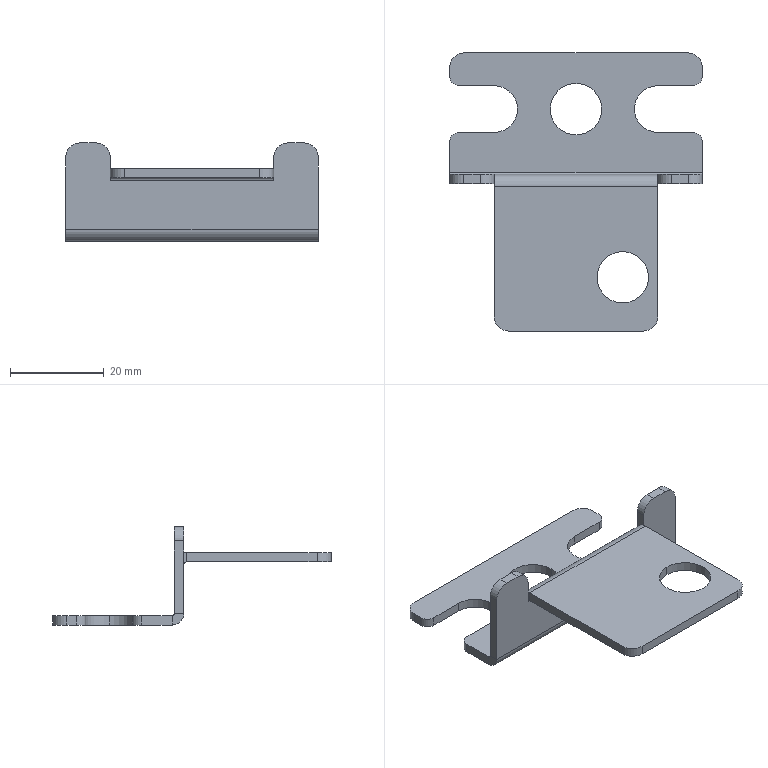Part | SolidWorks | features Fillet 3, EdgeFlange 2, ICE 2, Cut 1, FlatPattern 1, SMBaseFlange 1, SheetMetal 1 | 1 solid | 51 faces | box 54 x 59.5 x 21 mm | volume 5826 mm3 | plane 28 | cylinder 23 | commonest cylinder face diameters 6 x8 4 x4 11 x4 10 x3 1 x2 5 x2
STEP:
#1=CARTESIAN_POINT('',(10.,-28.5,13.5));
#2=VERTEX_POINT('',#1);
#3=CARTESIAN_POINT('',(10.,-39.5,13.5));
#4=VERTEX_POINT('',#3);
#5=CARTESIAN_POINT('',(10.,-34.,13.5));
#6=DIRECTION('',(0.,0.,1.));
#7=DIRECTION('',(0.,-1.,0.));
#8=AXIS2_PLACEMENT_3D('',#5,#6,#7);
#9=CIRCLE('',#8,5.5);
#10=EDGE_CURVE('',#2,#4,#9,.T.);
#11=ORIENTED_EDGE('',*,*,#10,.T.);
#12=CARTESIAN_POINT('',(10.,-39.5,11.5));
#13=VERTEX_POINT('',#12);
#14=CARTESIAN_POINT('',(10.,-39.5,21.5));
#15=DIRECTION('',(0.,0.,-1.));
#16=VECTOR('',#15,1000.);
#17=LINE('',#14,#16);
#18=EDGE_CURVE('',#4,#13,#17,.T.);
#19=ORIENTED_EDGE('',*,*,#18,.T.);
#20=CARTESIAN_POINT('',(10.,-28.5,11.5));
#21=VERTEX_POINT('',#20);
#22=CARTESIAN_POINT('',(10.,-34.,11.5));
#23=DIRECTION('',(0.,0.,-1.));
#24=DIRECTION('',(0.,1.,0.));
#25=AXIS2_PLACEMENT_3D('',#22,#23,#24);
#26=CIRCLE('',#25,5.5);
#27=EDGE_CURVE('',#13,#21,#26,.T.);
#28=ORIENTED_EDGE('',*,*,#27,.T.);
#29=CARTESIAN_POINT('',(10.,-28.5,21.5));
#30=DIRECTION('',(0.,0.,-1.));
#31=VECTOR('',#30,1000.);
#32=LINE('',#29,#31);
#33=EDGE_CURVE('',#2,#21,#32,.T.);
#34=ORIENTED_EDGE('',*,*,#33,.F.);
#35=EDGE_LOOP('',(#11,#19,#28,#34));
#36=FACE_OUTER_BOUND('',#35,.T.);
#37=CARTESIAN_POINT('',(10.,-34.,21.5));
#38=DIRECTION('',(0.,0.,-1.));
#39=DIRECTION('',(0.,1.,0.));
#40=AXIS2_PLACEMENT_3D('',#37,#38,#39);
#41=CYLINDRICAL_SURFACE('',#40,5.5);
#42=ADVANCED_FACE('',(#36),#41,.F.);
#43=CARTESIAN_POINT('',(-5.5,2.,-2.));
#44=VERTEX_POINT('',#43);
#45=CARTESIAN_POINT('',(5.5,2.,-2.));
#46=VERTEX_POINT('',#45);
#47=CARTESIAN_POINT('',(0.,2.,-2.));
#48=DIRECTION('',(0.,0.,1.));
#49=DIRECTION('',(1.,0.,0.));
#50=AXIS2_PLACEMENT_3D('',#47,#48,#49);
#51=CIRCLE('',#50,5.5);
#52=EDGE_CURVE('',#44,#46,#51,.T.);
#53=ORIENTED_EDGE('',*,*,#52,.F.);
#54=CARTESIAN_POINT('',(-5.5,2.,0.));
#55=VERTEX_POINT('',#54);
#56=CARTESIAN_POINT('',(-5.5,2.,-10.));
#57=DIRECTION('',(0.,0.,1.));
#58=VECTOR('',#57,1000.);
#59=LINE('',#56,#58);
#60=EDGE_CURVE('',#44,#55,#59,.T.);
#61=ORIENTED_EDGE('',*,*,#60,.T.);
#62=CARTESIAN_POINT('',(5.5,2.,0.));
#63=VERTEX_POINT('',#62);
#64=CARTESIAN_POINT('',(0.,2.,0.));
#65=DIRECTION('',(0.,0.,1.));
#66=DIRECTION('',(1.,0.,0.));
#67=AXIS2_PLACEMENT_3D('',#64,#65,#66);
#68=CIRCLE('',#67,5.5);
#69=EDGE_CURVE('',#55,#63,#68,.T.);
#70=ORIENTED_EDGE('',*,*,#69,.T.);
#71=CARTESIAN_POINT('',(5.5,2.,-10.));
#72=DIRECTION('',(0.,0.,1.));
#73=VECTOR('',#72,1000.);
#74=LINE('',#71,#73);
#75=EDGE_CURVE('',#46,#63,#74,.T.);
#76=ORIENTED_EDGE('',*,*,#75,.F.);
#77=EDGE_LOOP('',(#53,#61,#70,#76));
#78=FACE_OUTER_BOUND('',#77,.T.);
#79=CARTESIAN_POINT('',(0.,2.,-10.));
#80=DIRECTION('',(0.,0.,1.));
#81=DIRECTION('',(1.,0.,0.));
#82=AXIS2_PLACEMENT_3D('',#79,#80,#81);
#83=CYLINDRICAL_SURFACE('',#82,5.5);
#84=ADVANCED_FACE('',(#78),#83,.F.);
#85=CARTESIAN_POINT('',(-12.5,2.,-2.));
#86=VERTEX_POINT('',#85);
#87=CARTESIAN_POINT('',(-17.5,7.,-2.));
#88=VERTEX_POINT('',#87);
#89=CARTESIAN_POINT('',(-17.5,2.,-2.));
#90=DIRECTION('',(0.,0.,1.));
#91=DIRECTION('',(1.,0.,0.));
#92=AXIS2_PLACEMENT_3D('',#89,#90,#91);
#93=CIRCLE('',#92,5.);
#94=EDGE_CURVE('',#86,#88,#93,.T.);
#95=ORIENTED_EDGE('',*,*,#94,.F.);
#96=CARTESIAN_POINT('',(-12.5,2.,0.));
#97=VERTEX_POINT('',#96);
#98=CARTESIAN_POINT('',(-12.5,2.,-10.));
#99=DIRECTION('',(0.,0.,1.));
#100=VECTOR('',#99,1000.);
#101=LINE('',#98,#100);
#102=EDGE_CURVE('',#86,#97,#101,.T.);
#103=ORIENTED_EDGE('',*,*,#102,.T.);
#104=CARTESIAN_POINT('',(-17.5,7.,0.));
#105=VERTEX_POINT('',#104);
#106=CARTESIAN_POINT('',(-17.5,2.,0.));
#107=DIRECTION('',(0.,0.,1.));
#108=DIRECTION('',(-1.,0.,0.));
#109=AXIS2_PLACEMENT_3D('',#106,#107,#108);
#110=CIRCLE('',#109,5.);
#111=EDGE_CURVE('',#97,#105,#110,.T.);
#112=ORIENTED_EDGE('',*,*,#111,.T.);
#113=CARTESIAN_POINT('',(-17.5,7.,-10.));
#114=DIRECTION('',(0.,0.,1.));
#115=VECTOR('',#114,1000.);
#116=LINE('',#113,#115);
#117=EDGE_CURVE('',#88,#105,#116,.T.);
#118=ORIENTED_EDGE('',*,*,#117,.F.);
#119=EDGE_LOOP('',(#95,#103,#112,#118));
#120=FACE_OUTER_BOUND('',#119,.T.);
#121=CARTESIAN_POINT('',(-17.5,2.,-10.));
#122=DIRECTION('',(0.,0.,1.));
#123=DIRECTION('',(1.,0.,0.));
#124=AXIS2_PLACEMENT_3D('',#121,#122,#123);
#125=CYLINDRICAL_SURFACE('',#124,5.);
#126=ADVANCED_FACE('',(#120),#125,.F.);
#127=CARTESIAN_POINT('',(27.,9.,0.));
#128=VERTEX_POINT('',#127);
#129=CARTESIAN_POINT('',(27.,11.,0.));
#130=VERTEX_POINT('',#129);
#131=CARTESIAN_POINT('',(27.,14.,0.));
#132=DIRECTION('',(0.,1.,0.));
#133=VECTOR('',#132,1000.);
#134=LINE('',#131,#133);
#135=EDGE_CURVE('',#128,#130,#134,.T.);
#136=ORIENTED_EDGE('',*,*,#135,.F.);
#137=CARTESIAN_POINT('',(27.,9.,-2.));
#138=VERTEX_POINT('',#137);
#139=CARTESIAN_POINT('',(27.,9.,-2.));
#140=DIRECTION('',(0.,0.,-1.));
#141=VECTOR('',#140,1000.);
#142=LINE('',#139,#141);
#143=EDGE_CURVE('',#128,#138,#142,.T.);
#144=ORIENTED_EDGE('',*,*,#143,.T.);
#145=CARTESIAN_POINT('',(27.,11.,-2.));
#146=VERTEX_POINT('',#145);
#147=CARTESIAN_POINT('',(27.,14.,-2.));
#148=DIRECTION('',(0.,1.,0.));
#149=VECTOR('',#148,1000.);
#150=LINE('',#147,#149);
#151=EDGE_CURVE('',#138,#146,#150,.T.);
#152=ORIENTED_EDGE('',*,*,#151,.T.);
#153=CARTESIAN_POINT('',(27.,11.,-2.));
#154=DIRECTION('',(0.,0.,1.));
#155=VECTOR('',#154,1000.);
#156=LINE('',#153,#155);
#157=EDGE_CURVE('',#146,#130,#156,.T.);
#158=ORIENTED_EDGE('',*,*,#157,.T.);
#159=EDGE_LOOP('',(#136,#144,#152,#158));
#160=FACE_OUTER_BOUND('',#159,.T.);
#161=CARTESIAN_POINT('',(27.,14.,-2.));
#162=DIRECTION('',(1.,0.,0.));
#163=DIRECTION('',(0.,1.,0.));
#164=AXIS2_PLACEMENT_3D('',#161,#162,#163);
#165=PLANE('',#164);
#166=ADVANCED_FACE('',(#160),#165,.T.);
#167=CARTESIAN_POINT('',(-27.,-5.,0.));
#168=VERTEX_POINT('',#167);
#169=CARTESIAN_POINT('',(-27.,-11.5,0.));
#170=VERTEX_POINT('',#169);
#171=CARTESIAN_POINT('',(-27.,14.,0.));
#172=DIRECTION('',(0.,-1.,0.));
#173=VECTOR('',#172,1000.);
#174=LINE('',#171,#173);
#175=EDGE_CURVE('',#168,#170,#174,.T.);
#176=ORIENTED_EDGE('',*,*,#175,.F.);
#177=CARTESIAN_POINT('',(-27.,-5.,-2.));
#178=VERTEX_POINT('',#177);
#179=CARTESIAN_POINT('',(-27.,-5.,-2.));
#180=DIRECTION('',(0.,0.,-1.));
#181=VECTOR('',#180,1000.);
#182=LINE('',#179,#181);
#183=EDGE_CURVE('',#168,#178,#182,.T.);
#184=ORIENTED_EDGE('',*,*,#183,.T.);
#185=CARTESIAN_POINT('',(-27.,-11.5,-2.));
#186=VERTEX_POINT('',#185);
#187=CARTESIAN_POINT('',(-27.,14.,-2.));
#188=DIRECTION('',(0.,-1.,0.));
#189=VECTOR('',#188,1000.);
#190=LINE('',#187,#189);
#191=EDGE_CURVE('',#178,#186,#190,.T.);
#192=ORIENTED_EDGE('',*,*,#191,.T.);
#193=CARTESIAN_POINT('',(-27.,-11.5,0.));
#194=DIRECTION('',(0.,0.,-1.));
#195=VECTOR('',#194,1000.);
#196=LINE('',#193,#195);
#197=EDGE_CURVE('',#170,#186,#196,.T.);
#198=ORIENTED_EDGE('',*,*,#197,.F.);
#199=EDGE_LOOP('',(#176,#184,#192,#198));
#200=FACE_OUTER_BOUND('',#199,.T.);
#201=CARTESIAN_POINT('',(-27.,14.,-2.));
#202=DIRECTION('',(-1.,0.,0.));
#203=DIRECTION('',(0.,0.,1.));
#204=AXIS2_PLACEMENT_3D('',#201,#202,#203);
#205=PLANE('',#204);
#206=ADVANCED_FACE('',(#200),#205,.T.);
#207=CARTESIAN_POINT('',(-17.5,-14.,16.));
#208=VERTEX_POINT('',#207);
#209=CARTESIAN_POINT('',(-17.5,-14.,13.449));
#210=VERTEX_POINT('',#209);
#211=CARTESIAN_POINT('',(-17.5,-14.,0.));
#212=DIRECTION('',(0.,0.,-1.));
#213=VECTOR('',#212,1000.);
#214=LINE('',#211,#213);
#215=EDGE_CURVE('',#208,#210,#214,.T.);
#216=ORIENTED_EDGE('',*,*,#215,.F.);
#217=CARTESIAN_POINT('',(-20.5,-14.,19.));
#218=VERTEX_POINT('',#217);
#219=CARTESIAN_POINT('',(-20.5,-14.,16.));
#220=DIRECTION('',(0.,-1.,0.));
#221=DIRECTION('',(0.,0.,-1.));
#222=AXIS2_PLACEMENT_3D('',#219,#220,#221);
#223=CIRCLE('',#222,3.);
#224=EDGE_CURVE('',#208,#218,#223,.T.);
#225=ORIENTED_EDGE('',*,*,#224,.T.);
#226=CARTESIAN_POINT('',(-24.,-14.,19.));
#227=VERTEX_POINT('',#226);
#228=CARTESIAN_POINT('',(27.,-14.,19.));
#229=DIRECTION('',(1.,0.,0.));
#230=VECTOR('',#229,1000.);
#231=LINE('',#228,#230);
#232=EDGE_CURVE('',#227,#218,#231,.T.);
#233=ORIENTED_EDGE('',*,*,#232,.F.);
#234=CARTESIAN_POINT('',(-27.,-14.,16.));
#235=VERTEX_POINT('',#234);
#236=CARTESIAN_POINT('',(-24.,-14.,16.));
#237=DIRECTION('',(0.,-1.,0.));
#238=DIRECTION('',(0.,0.,-1.));
#239=AXIS2_PLACEMENT_3D('',#236,#237,#238);
#240=CIRCLE('',#239,3.);
#241=EDGE_CURVE('',#227,#235,#240,.T.);
#242=ORIENTED_EDGE('',*,*,#241,.T.);
#243=CARTESIAN_POINT('',(-27.,-14.,0.5));
#244=VERTEX_POINT('',#243);
#245=CARTESIAN_POINT('',(-27.,-14.,19.));
#246=DIRECTION('',(0.,0.,1.));
#247=VECTOR('',#246,1000.);
#248=LINE('',#245,#247);
#249=EDGE_CURVE('',#244,#235,#248,.T.);
#250=ORIENTED_EDGE('',*,*,#249,.F.);
#251=CARTESIAN_POINT('',(27.,-14.,0.5));
#252=VERTEX_POINT('',#251);
#253=CARTESIAN_POINT('',(0.,-14.,0.5));
#254=DIRECTION('',(1.,0.,0.));
#255=VECTOR('',#254,1000.);
#256=LINE('',#253,#255);
#257=EDGE_CURVE('',#244,#252,#256,.T.);
#258=ORIENTED_EDGE('',*,*,#257,.T.);
#259=CARTESIAN_POINT('',(27.,-14.,16.));
#260=VERTEX_POINT('',#259);
#261=CARTESIAN_POINT('',(27.,-14.,0.));
#262=DIRECTION('',(0.,0.,-1.));
#263=VECTOR('',#262,1000.);
#264=LINE('',#261,#263);
#265=EDGE_CURVE('',#260,#252,#264,.T.);
#266=ORIENTED_EDGE('',*,*,#265,.F.);
#267=CARTESIAN_POINT('',(24.,-14.,19.));
#268=VERTEX_POINT('',#267);
#269=CARTESIAN_POINT('',(24.,-14.,16.));
#270=DIRECTION('',(0.,-1.,0.));
#271=DIRECTION('',(0.,0.,-1.));
#272=AXIS2_PLACEMENT_3D('',#269,#270,#271);
#273=CIRCLE('',#272,3.);
#274=EDGE_CURVE('',#260,#268,#273,.T.);
#275=ORIENTED_EDGE('',*,*,#274,.T.);
#276=CARTESIAN_POINT('',(20.5,-14.,19.));
#277=VERTEX_POINT('',#276);
#278=CARTESIAN_POINT('',(27.,-14.,19.));
#279=DIRECTION('',(1.,0.,0.));
#280=VECTOR('',#279,1000.);
#281=LINE('',#278,#280);
#282=EDGE_CURVE('',#277,#268,#281,.T.);
#283=ORIENTED_EDGE('',*,*,#282,.F.);
#284=CARTESIAN_POINT('',(17.5,-14.,16.));
#285=VERTEX_POINT('',#284);
#286=CARTESIAN_POINT('',(20.5,-14.,16.));
#287=DIRECTION('',(0.,-1.,0.));
#288=DIRECTION('',(0.,0.,-1.));
#289=AXIS2_PLACEMENT_3D('',#286,#287,#288);
#290=CIRCLE('',#289,3.);
#291=EDGE_CURVE('',#277,#285,#290,.T.);
#292=ORIENTED_EDGE('',*,*,#291,.T.);
#293=CARTESIAN_POINT('',(17.5,-14.,13.449));
#294=VERTEX_POINT('',#293);
#295=CARTESIAN_POINT('',(17.5,-14.,0.));
#296=DIRECTION('',(0.,0.,1.));
#297=VECTOR('',#296,1000.);
#298=LINE('',#295,#297);
#299=EDGE_CURVE('',#294,#285,#298,.T.);
#300=ORIENTED_EDGE('',*,*,#299,.F.);
#301=CARTESIAN_POINT('',(17.5,-14.,11.));
#302=VERTEX_POINT('',#301);
#303=CARTESIAN_POINT('',(17.5,-14.,0.));
#304=DIRECTION('',(0.,0.,1.));
#305=VECTOR('',#304,1000.);
#306=LINE('',#303,#305);
#307=EDGE_CURVE('',#302,#294,#306,.T.);
#308=ORIENTED_EDGE('',*,*,#307,.F.);
#309=CARTESIAN_POINT('',(-17.5,-14.,11.));
#310=VERTEX_POINT('',#309);
#311=CARTESIAN_POINT('',(-17.5,-14.,11.));
#312=DIRECTION('',(1.,0.,0.));
#313=VECTOR('',#312,1000.);
#314=LINE('',#311,#313);
#315=EDGE_CURVE('',#310,#302,#314,.T.);
#316=ORIENTED_EDGE('',*,*,#315,.F.);
#317=CARTESIAN_POINT('',(-17.5,-14.,0.));
#318=DIRECTION('',(0.,0.,-1.));
#319=VECTOR('',#318,1000.);
#320=LINE('',#317,#319);
#321=EDGE_CURVE('',#210,#310,#320,.T.);
#322=ORIENTED_EDGE('',*,*,#321,.F.);
#323=EDGE_LOOP('',(#216,#225,#233,#242,#250,#258,#266,#275,#283,#292,#300,#308,#316,#322));
#324=FACE_OUTER_BOUND('',#323,.T.);
#325=CARTESIAN_POINT('',(0.,-14.,0.));
#326=DIRECTION('',(0.,-1.,0.));
#327=DIRECTION('',(0.,0.,-1.));
#328=AXIS2_PLACEMENT_3D('',#325,#326,#327);
#329=PLANE('',#328);
#330=ADVANCED_FACE('',(#324),#329,.T.);
#331=CARTESIAN_POINT('',(-24.,-12.,19.));
#332=VERTEX_POINT('',#331);
#333=CARTESIAN_POINT('',(-20.5,-12.,19.));
#334=VERTEX_POINT('',#333);
#335=CARTESIAN_POINT('',(0.,-12.,19.));
#336=DIRECTION('',(1.,0.,0.));
#337=VECTOR('',#336,1000.);
#338=LINE('',#335,#337);
#339=EDGE_CURVE('',#332,#334,#338,.T.);
#340=ORIENTED_EDGE('',*,*,#339,.T.);
#341=CARTESIAN_POINT('',(-17.5,-12.,16.));
#342=VERTEX_POINT('',#341);
#343=CARTESIAN_POINT('',(-20.5,-12.,16.));
#344=DIRECTION('',(0.,1.,0.));
#345=DIRECTION('',(0.,0.,-1.));
#346=AXIS2_PLACEMENT_3D('',#343,#344,#345);
#347=CIRCLE('',#346,3.);
#348=EDGE_CURVE('',#334,#342,#347,.T.);
#349=ORIENTED_EDGE('',*,*,#348,.T.);
#350=CARTESIAN_POINT('',(-17.5,-12.,11.));
#351=VERTEX_POINT('',#350);
#352=CARTESIAN_POINT('',(-17.5,-12.,24.5));
#353=DIRECTION('',(0.,0.,1.));
#354=VECTOR('',#353,1000.);
#355=LINE('',#352,#354);
#356=EDGE_CURVE('',#351,#342,#355,.T.);
#357=ORIENTED_EDGE('',*,*,#356,.F.);
#358=CARTESIAN_POINT('',(17.5,-12.,11.));
#359=VERTEX_POINT('',#358);
#360=CARTESIAN_POINT('',(-17.5,-12.,11.));
#361=DIRECTION('',(1.,0.,0.));
#362=VECTOR('',#361,1000.);
#363=LINE('',#360,#362);
#364=EDGE_CURVE('',#351,#359,#363,.T.);
#365=ORIENTED_EDGE('',*,*,#364,.T.);
#366=CARTESIAN_POINT('',(17.5,-12.,16.));
#367=VERTEX_POINT('',#366);
#368=CARTESIAN_POINT('',(17.5,-12.,24.5));
#369=DIRECTION('',(0.,0.,-1.));
#370=VECTOR('',#369,1000.);
#371=LINE('',#368,#370);
#372=EDGE_CURVE('',#367,#359,#371,.T.);
#373=ORIENTED_EDGE('',*,*,#372,.F.);
#374=CARTESIAN_POINT('',(20.5,-12.,19.));
#375=VERTEX_POINT('',#374);
#376=CARTESIAN_POINT('',(20.5,-12.,16.));
#377=DIRECTION('',(0.,1.,0.));
#378=DIRECTION('',(0.,0.,-1.));
#379=AXIS2_PLACEMENT_3D('',#376,#377,#378);
#380=CIRCLE('',#379,3.);
#381=EDGE_CURVE('',#367,#375,#380,.T.);
#382=ORIENTED_EDGE('',*,*,#381,.T.);
#383=CARTESIAN_POINT('',(24.,-12.,19.));
#384=VERTEX_POINT('',#383);
#385=CARTESIAN_POINT('',(0.,-12.,19.));
#386=DIRECTION('',(1.,0.,0.));
#387=VECTOR('',#386,1000.);
#388=LINE('',#385,#387);
#389=EDGE_CURVE('',#375,#384,#388,.T.);
#390=ORIENTED_EDGE('',*,*,#389,.T.);
#391=CARTESIAN_POINT('',(27.,-12.,16.));
#392=VERTEX_POINT('',#391);
#393=CARTESIAN_POINT('',(24.,-12.,16.));
#394=DIRECTION('',(0.,1.,0.));
#395=DIRECTION('',(0.,0.,-1.));
#396=AXIS2_PLACEMENT_3D('',#393,#394,#395);
#397=CIRCLE('',#396,3.);
#398=EDGE_CURVE('',#384,#392,#397,.T.);
#399=ORIENTED_EDGE('',*,*,#398,.T.);
#400=CARTESIAN_POINT('',(27.,-12.,0.5));
#401=VERTEX_POINT('',#400);
#402=CARTESIAN_POINT('',(27.,-12.,0.));
#403=DIRECTION('',(0.,0.,-1.));
#404=VECTOR('',#403,1000.);
#405=LINE('',#402,#404);
#406=EDGE_CURVE('',#392,#401,#405,.T.);
#407=ORIENTED_EDGE('',*,*,#406,.T.);
#408=CARTESIAN_POINT('',(-27.,-12.,0.5));
#409=VERTEX_POINT('',#408);
#410=CARTESIAN_POINT('',(-27.,-12.,0.5));
#411=DIRECTION('',(1.,0.,0.));
#412=VECTOR('',#411,1000.);
#413=LINE('',#410,#412);
#414=EDGE_CURVE('',#409,#401,#413,.T.);
#415=ORIENTED_EDGE('',*,*,#414,.F.);
#416=CARTESIAN_POINT('',(-27.,-12.,16.));
#417=VERTEX_POINT('',#416);
#418=CARTESIAN_POINT('',(-27.,-12.,0.));
#419=DIRECTION('',(0.,0.,1.));
#420=VECTOR('',#419,1000.);
#421=LINE('',#418,#420);
#422=EDGE_CURVE('',#409,#417,#421,.T.);
#423=ORIENTED_EDGE('',*,*,#422,.T.);
#424=CARTESIAN_POINT('',(-24.,-12.,16.));
#425=DIRECTION('',(0.,1.,0.));
#426=DIRECTION('',(0.,0.,-1.));
#427=AXIS2_PLACEMENT_3D('',#424,#425,#426);
#428=CIRCLE('',#427,3.);
#429=EDGE_CURVE('',#417,#332,#428,.T.);
#430=ORIENTED_EDGE('',*,*,#429,.T.);
#431=EDGE_LOOP('',(#340,#349,#357,#365,#373,#382,#390,#399,#407,#415,#423,#430));
#432=FACE_OUTER_BOUND('',#431,.T.);
#433=CARTESIAN_POINT('',(0.,-12.,0.));
#434=DIRECTION('',(0.,-1.,0.));
#435=DIRECTION('',(0.,0.,-1.));
#436=AXIS2_PLACEMENT_3D('',#433,#434,#435);
#437=PLANE('',#436);
#438=ADVANCED_FACE('',(#432),#437,.F.);
#439=ORIENTED_EDGE('',*,*,#282,.T.);
#440=CARTESIAN_POINT('',(24.,-14.,19.));
#441=DIRECTION('',(0.,1.,0.));
#442=VECTOR('',#441,1000.);
#443=LINE('',#440,#442);
#444=EDGE_CURVE('',#268,#384,#443,.T.);
#445=ORIENTED_EDGE('',*,*,#444,.T.);
#446=ORIENTED_EDGE('',*,*,#389,.F.);
#447=CARTESIAN_POINT('',(20.5,-14.,19.));
#448=DIRECTION('',(0.,-1.,0.));
#449=VECTOR('',#448,1000.);
#450=LINE('',#447,#449);
#451=EDGE_CURVE('',#375,#277,#450,.T.);
#452=ORIENTED_EDGE('',*,*,#451,.T.);
#453=EDGE_LOOP('',(#439,#445,#446,#452));
#454=FACE_OUTER_BOUND('',#453,.T.);
#455=CARTESIAN_POINT('',(27.,-14.,19.));
#456=DIRECTION('',(0.,0.,1.));
#457=DIRECTION('',(0.,-1.,0.));
#458=AXIS2_PLACEMENT_3D('',#455,#456,#457);
#459=PLANE('',#458);
#460=ADVANCED_FACE('',(#454),#459,.T.);
#461=CARTESIAN_POINT('',(27.,-11.5,-2.));
#462=VERTEX_POINT('',#461);
#463=CARTESIAN_POINT('',(27.,-5.,-2.));
#464=VERTEX_POINT('',#463);
#465=CARTESIAN_POINT('',(27.,14.,-2.));
#466=DIRECTION('',(0.,1.,0.));
#467=VECTOR('',#466,1000.);
#468=LINE('',#465,#467);
#469=EDGE_CURVE('',#462,#464,#468,.T.);
#470=ORIENTED_EDGE('',*,*,#469,.T.);
#471=CARTESIAN_POINT('',(27.,-5.,0.));
#472=VERTEX_POINT('',#471);
#473=CARTESIAN_POINT('',(27.,-5.,0.));
#474=DIRECTION('',(0.,0.,1.));
#475=VECTOR('',#474,1000.);
#476=LINE('',#473,#475);
#477=EDGE_CURVE('',#464,#472,#476,.T.);
#478=ORIENTED_EDGE('',*,*,#477,.T.);
#479=CARTESIAN_POINT('',(27.,-11.5,0.));
#480=VERTEX_POINT('',#479);
#481=CARTESIAN_POINT('',(27.,14.,0.));
#482=DIRECTION('',(0.,1.,0.));
#483=VECTOR('',#482,1000.);
#484=LINE('',#481,#483);
#485=EDGE_CURVE('',#480,#472,#484,.T.);
#486=ORIENTED_EDGE('',*,*,#485,.F.);
#487=CARTESIAN_POINT('',(27.,-11.5,0.));
#488=DIRECTION('',(0.,0.,-1.));
#489=VECTOR('',#488,1000.);
#490=LINE('',#487,#489);
#491=EDGE_CURVE('',#480,#462,#490,.T.);
#492=ORIENTED_EDGE('',*,*,#491,.T.);
#493=EDGE_LOOP('',(#470,#478,#486,#492));
#494=FACE_OUTER_BOUND('',#493,.T.);
#495=CARTESIAN_POINT('',(27.,14.,-2.));
#496=DIRECTION('',(1.,0.,0.));
#497=DIRECTION('',(0.,1.,0.));
#498=AXIS2_PLACEMENT_3D('',#495,#496,#497);
#499=PLANE('',#498);
#500=ADVANCED_FACE('',(#494),#499,.T.);
#501=CARTESIAN_POINT('',(0.,2.,-2.));
#502=DIRECTION('',(0.,0.,1.));
#503=DIRECTION('',(1.,0.,0.));
#504=AXIS2_PLACEMENT_3D('',#501,#502,#503);
#505=CIRCLE('',#504,5.5);
#506=EDGE_CURVE('',#46,#44,#505,.T.);
#507=ORIENTED_EDGE('',*,*,#506,.T.);
#508=ORIENTED_EDGE('',*,*,#52,.T.);
#509=EDGE_LOOP('',(#507,#508));
#510=FACE_BOUND('',#509,.T.);
#511=ORIENTED_EDGE('',*,*,#191,.F.);
#512=CARTESIAN_POINT('',(-25.,-3.,-2.));
#513=VERTEX_POINT('',#512);
#514=CARTESIAN_POINT('',(-25.,-5.,-2.));
#515=DIRECTION('',(0.,0.,-1.));
#516=DIRECTION('',(1.,0.,0.));
#517=AXIS2_PLACEMENT_3D('',#514,#515,#516);
#518=CIRCLE('',#517,2.);
#519=EDGE_CURVE('',#178,#513,#518,.T.);
#520=ORIENTED_EDGE('',*,*,#519,.T.);
#521=CARTESIAN_POINT('',(-17.5,-3.,-2.));
#522=VERTEX_POINT('',#521);
#523=CARTESIAN_POINT('',(0.,-3.,-2.));
#524=DIRECTION('',(1.,0.,0.));
#525=VECTOR('',#524,1000.);
#526=LINE('',#523,#525);
#527=EDGE_CURVE('',#513,#522,#526,.T.);
#528=ORIENTED_EDGE('',*,*,#527,.T.);
#529=CARTESIAN_POINT('',(-17.5,2.,-2.));
#530=DIRECTION('',(0.,0.,1.));
#531=DIRECTION('',(1.,0.,0.));
#532=AXIS2_PLACEMENT_3D('',#529,#530,#531);
#533=CIRCLE('',#532,5.);
#534=EDGE_CURVE('',#522,#86,#533,.T.);
#535=ORIENTED_EDGE('',*,*,#534,.T.);
#536=ORIENTED_EDGE('',*,*,#94,.T.);
#537=CARTESIAN_POINT('',(-25.,7.,-2.));
#538=VERTEX_POINT('',#537);
#539=CARTESIAN_POINT('',(0.,7.,-2.));
#540=DIRECTION('',(-1.,0.,0.));
#541=VECTOR('',#540,1000.);
#542=LINE('',#539,#541);
#543=EDGE_CURVE('',#88,#538,#542,.T.);
#544=ORIENTED_EDGE('',*,*,#543,.T.);
#545=CARTESIAN_POINT('',(-27.,9.,-2.));
#546=VERTEX_POINT('',#545);
#547=CARTESIAN_POINT('',(-25.,9.,-2.));
#548=DIRECTION('',(0.,0.,-1.));
#549=DIRECTION('',(1.,0.,0.));
#550=AXIS2_PLACEMENT_3D('',#547,#548,#549);
#551=CIRCLE('',#550,2.);
#552=EDGE_CURVE('',#538,#546,#551,.T.);
#553=ORIENTED_EDGE('',*,*,#552,.T.);
#554=CARTESIAN_POINT('',(-27.,11.,-2.));
#555=VERTEX_POINT('',#554);
#556=CARTESIAN_POINT('',(-27.,14.,-2.));
#557=DIRECTION('',(0.,-1.,0.));
#558=VECTOR('',#557,1000.);
#559=LINE('',#556,#558);
#560=EDGE_CURVE('',#555,#546,#559,.T.);
#561=ORIENTED_EDGE('',*,*,#560,.F.);
#562=CARTESIAN_POINT('',(-24.,14.,-2.));
#563=VERTEX_POINT('',#562);
#564=CARTESIAN_POINT('',(-24.,11.,-2.));
#565=DIRECTION('',(0.,0.,-1.));
#566=DIRECTION('',(1.,0.,0.));
#567=AXIS2_PLACEMENT_3D('',#564,#565,#566);
#568=CIRCLE('',#567,3.);
#569=EDGE_CURVE('',#555,#563,#568,.T.);
#570=ORIENTED_EDGE('',*,*,#569,.T.);
#571=CARTESIAN_POINT('',(24.,14.,-2.));
#572=VERTEX_POINT('',#571);
#573=CARTESIAN_POINT('',(-27.,14.,-2.));
#574=DIRECTION('',(-1.,0.,0.));
#575=VECTOR('',#574,1000.);
#576=LINE('',#573,#575);
#577=EDGE_CURVE('',#572,#563,#576,.T.);
#578=ORIENTED_EDGE('',*,*,#577,.F.);
#579=CARTESIAN_POINT('',(24.,11.,-2.));
#580=DIRECTION('',(0.,0.,-1.));
#581=DIRECTION('',(1.,0.,0.));
#582=AXIS2_PLACEMENT_3D('',#579,#580,#581);
#583=CIRCLE('',#582,3.);
#584=EDGE_CURVE('',#572,#146,#583,.T.);
#585=ORIENTED_EDGE('',*,*,#584,.T.);
#586=ORIENTED_EDGE('',*,*,#151,.F.);
#587=CARTESIAN_POINT('',(25.,7.,-2.));
#588=VERTEX_POINT('',#587);
#589=CARTESIAN_POINT('',(25.,9.,-2.));
#590=DIRECTION('',(0.,0.,-1.));
#591=DIRECTION('',(1.,0.,0.));
#592=AXIS2_PLACEMENT_3D('',#589,#590,#591);
#593=CIRCLE('',#592,2.);
#594=EDGE_CURVE('',#138,#588,#593,.T.);
#595=ORIENTED_EDGE('',*,*,#594,.T.);
#596=CARTESIAN_POINT('',(17.5,7.,-2.));
#597=VERTEX_POINT('',#596);
#598=CARTESIAN_POINT('',(0.,7.,-2.));
#599=DIRECTION('',(-1.,0.,0.));
#600=VECTOR('',#599,1000.);
#601=LINE('',#598,#600);
#602=EDGE_CURVE('',#588,#597,#601,.T.);
#603=ORIENTED_EDGE('',*,*,#602,.T.);
#604=CARTESIAN_POINT('',(17.5,-3.,-2.));
#605=VERTEX_POINT('',#604);
#606=CARTESIAN_POINT('',(17.5,2.,-2.));
#607=DIRECTION('',(0.,0.,1.));
#608=DIRECTION('',(1.,0.,0.));
#609=AXIS2_PLACEMENT_3D('',#606,#607,#608);
#610=CIRCLE('',#609,5.);
#611=EDGE_CURVE('',#597,#605,#610,.T.);
#612=ORIENTED_EDGE('',*,*,#611,.T.);
#613=CARTESIAN_POINT('',(25.,-3.,-2.));
#614=VERTEX_POINT('',#613);
#615=CARTESIAN_POINT('',(0.,-3.,-2.));
#616=DIRECTION('',(1.,0.,0.));
#617=VECTOR('',#616,1000.);
#618=LINE('',#615,#617);
#619=EDGE_CURVE('',#605,#614,#618,.T.);
#620=ORIENTED_EDGE('',*,*,#619,.T.);
#621=CARTESIAN_POINT('',(25.,-5.,-2.));
#622=DIRECTION('',(0.,0.,-1.));
#623=DIRECTION('',(1.,0.,0.));
#624=AXIS2_PLACEMENT_3D('',#621,#622,#623);
#625=CIRCLE('',#624,2.);
#626=EDGE_CURVE('',#614,#464,#625,.T.);
#627=ORIENTED_EDGE('',*,*,#626,.T.);
#628=ORIENTED_EDGE('',*,*,#469,.F.);
#629=CARTESIAN_POINT('',(27.,-11.5,-2.));
#630=DIRECTION('',(-1.,0.,0.));
#631=VECTOR('',#630,1000.);
#632=LINE('',#629,#631);
#633=EDGE_CURVE('',#462,#186,#632,.T.);
#634=ORIENTED_EDGE('',*,*,#633,.T.);
#635=EDGE_LOOP('',(#511,#520,#528,#535,#536,#544,#553,#561,#570,#578,#585,#586,#595,#603,#612,#620,#627,#628,#634));
#636=FACE_OUTER_BOUND('',#635,.T.);
#637=CARTESIAN_POINT('',(0.,0.,-2.));
#638=DIRECTION('',(0.,0.,1.));
#639=DIRECTION('',(1.,0.,0.));
#640=AXIS2_PLACEMENT_3D('',#637,#638,#639);
#641=PLANE('',#640);
#642=ADVANCED_FACE('',(#510,#636),#641,.F.);
#643=CARTESIAN_POINT('',(-25.,-3.,0.));
#644=VERTEX_POINT('',#643);
#645=CARTESIAN_POINT('',(-17.5,-3.,0.));
#646=VERTEX_POINT('',#645);
#647=CARTESIAN_POINT('',(-17.5,-3.,0.));
#648=DIRECTION('',(1.,0.,0.));
#649=VECTOR('',#648,1000.);
#650=LINE('',#647,#649);
#651=EDGE_CURVE('',#644,#646,#650,.T.);
#652=ORIENTED_EDGE('',*,*,#651,.F.);
#653=CARTESIAN_POINT('',(-25.,-5.,0.));
#654=DIRECTION('',(0.,0.,1.));
#655=DIRECTION('',(1.,0.,0.));
#656=AXIS2_PLACEMENT_3D('',#653,#654,#655);
#657=CIRCLE('',#656,2.);
#658=EDGE_CURVE('',#644,#168,#657,.T.);
#659=ORIENTED_EDGE('',*,*,#658,.T.);
#660=ORIENTED_EDGE('',*,*,#175,.T.);
#661=CARTESIAN_POINT('',(27.,-11.5,0.));
#662=DIRECTION('',(-1.,0.,0.));
#663=VECTOR('',#662,1000.);
#664=LINE('',#661,#663);
#665=EDGE_CURVE('',#480,#170,#664,.T.);
#666=ORIENTED_EDGE('',*,*,#665,.F.);
#667=ORIENTED_EDGE('',*,*,#485,.T.);
#668=CARTESIAN_POINT('',(25.,-3.,0.));
#669=VERTEX_POINT('',#668);
#670=CARTESIAN_POINT('',(25.,-5.,0.));
#671=DIRECTION('',(0.,0.,1.));
#672=DIRECTION('',(1.,0.,0.));
#673=AXIS2_PLACEMENT_3D('',#670,#671,#672);
#674=CIRCLE('',#673,2.);
#675=EDGE_CURVE('',#472,#669,#674,.T.);
#676=ORIENTED_EDGE('',*,*,#675,.T.);
#677=CARTESIAN_POINT('',(17.5,-3.,0.));
#678=VERTEX_POINT('',#677);
#679=CARTESIAN_POINT('',(17.5,-3.,0.));
#680=DIRECTION('',(1.,0.,0.));
#681=VECTOR('',#680,1000.);
#682=LINE('',#679,#681);
#683=EDGE_CURVE('',#678,#669,#682,.T.);
#684=ORIENTED_EDGE('',*,*,#683,.F.);
#685=CARTESIAN_POINT('',(17.5,7.,0.));
#686=VERTEX_POINT('',#685);
#687=CARTESIAN_POINT('',(17.5,2.,0.));
#688=DIRECTION('',(0.,0.,1.));
#689=DIRECTION('',(1.,0.,0.));
#690=AXIS2_PLACEMENT_3D('',#687,#688,#689);
#691=CIRCLE('',#690,5.);
#692=EDGE_CURVE('',#686,#678,#691,.T.);
#693=ORIENTED_EDGE('',*,*,#692,.F.);
#694=CARTESIAN_POINT('',(25.,7.,0.));
#695=VERTEX_POINT('',#694);
#696=CARTESIAN_POINT('',(0.,7.,0.));
#697=DIRECTION('',(-1.,0.,0.));
#698=VECTOR('',#697,1000.);
#699=LINE('',#696,#698);
#700=EDGE_CURVE('',#695,#686,#699,.T.);
#701=ORIENTED_EDGE('',*,*,#700,.F.);
#702=CARTESIAN_POINT('',(25.,9.,0.));
#703=DIRECTION('',(0.,0.,1.));
#704=DIRECTION('',(1.,0.,0.));
#705=AXIS2_PLACEMENT_3D('',#702,#703,#704);
#706=CIRCLE('',#705,2.);
#707=EDGE_CURVE('',#695,#128,#706,.T.);
#708=ORIENTED_EDGE('',*,*,#707,.T.);
#709=ORIENTED_EDGE('',*,*,#135,.T.);
#710=CARTESIAN_POINT('',(24.,14.,0.));
#711=VERTEX_POINT('',#710);
#712=CARTESIAN_POINT('',(24.,11.,0.));
#713=DIRECTION('',(0.,0.,1.));
#714=DIRECTION('',(1.,0.,0.));
#715=AXIS2_PLACEMENT_3D('',#712,#713,#714);
#716=CIRCLE('',#715,3.);
#717=EDGE_CURVE('',#130,#711,#716,.T.);
#718=ORIENTED_EDGE('',*,*,#717,.T.);
#719=CARTESIAN_POINT('',(-24.,14.,0.));
#720=VERTEX_POINT('',#719);
#721=CARTESIAN_POINT('',(-27.,14.,0.));
#722=DIRECTION('',(-1.,0.,0.));
#723=VECTOR('',#722,1000.);
#724=LINE('',#721,#723);
#725=EDGE_CURVE('',#711,#720,#724,.T.);
#726=ORIENTED_EDGE('',*,*,#725,.T.);
#727=CARTESIAN_POINT('',(-27.,11.,0.));
#728=VERTEX_POINT('',#727);
#729=CARTESIAN_POINT('',(-24.,11.,0.));
#730=DIRECTION('',(0.,0.,1.));
#731=DIRECTION('',(1.,0.,0.));
#732=AXIS2_PLACEMENT_3D('',#729,#730,#731);
#733=CIRCLE('',#732,3.);
#734=EDGE_CURVE('',#720,#728,#733,.T.);
#735=ORIENTED_EDGE('',*,*,#734,.T.);
#736=CARTESIAN_POINT('',(-27.,9.,0.));
#737=VERTEX_POINT('',#736);
#738=CARTESIAN_POINT('',(-27.,14.,0.));
#739=DIRECTION('',(0.,-1.,0.));
#740=VECTOR('',#739,1000.);
#741=LINE('',#738,#740);
#742=EDGE_CURVE('',#728,#737,#741,.T.);
#743=ORIENTED_EDGE('',*,*,#742,.T.);
#744=CARTESIAN_POINT('',(-25.,7.,0.));
#745=VERTEX_POINT('',#744);
#746=CARTESIAN_POINT('',(-25.,9.,0.));
#747=DIRECTION('',(0.,0.,1.));
#748=DIRECTION('',(1.,0.,0.));
#749=AXIS2_PLACEMENT_3D('',#746,#747,#748);
#750=CIRCLE('',#749,2.);
#751=EDGE_CURVE('',#737,#745,#750,.T.);
#752=ORIENTED_EDGE('',*,*,#751,.T.);
#753=CARTESIAN_POINT('',(-17.5,7.,0.));
#754=DIRECTION('',(-1.,0.,0.));
#755=VECTOR('',#754,1000.);
#756=LINE('',#753,#755);
#757=EDGE_CURVE('',#105,#745,#756,.T.);
#758=ORIENTED_EDGE('',*,*,#757,.F.);
#759=ORIENTED_EDGE('',*,*,#111,.F.);
#760=CARTESIAN_POINT('',(-17.5,2.,0.));
#761=DIRECTION('',(0.,0.,1.));
#762=DIRECTION('',(-1.,0.,0.));
#763=AXIS2_PLACEMENT_3D('',#760,#761,#762);
#764=CIRCLE('',#763,5.);
#765=EDGE_CURVE('',#646,#97,#764,.T.);
#766=ORIENTED_EDGE('',*,*,#765,.F.);
#767=EDGE_LOOP('',(#652,#659,#660,#666,#667,#676,#684,#693,#701,#708,#709,#718,#726,#735,#743,#752,#758,#759,#766));
#768=FACE_OUTER_BOUND('',#767,.T.);
#769=CARTESIAN_POINT('',(0.,2.,0.));
#770=DIRECTION('',(0.,0.,1.));
#771=DIRECTION('',(1.,0.,0.));
#772=AXIS2_PLACEMENT_3D('',#769,#770,#771);
#773=CIRCLE('',#772,5.5);
#774=EDGE_CURVE('',#63,#55,#773,.T.);
#775=ORIENTED_EDGE('',*,*,#774,.F.);
#776=ORIENTED_EDGE('',*,*,#69,.F.);
#777=EDGE_LOOP('',(#775,#776));
#778=FACE_BOUND('',#777,.T.);
#779=CARTESIAN_POINT('',(0.,0.,0.));
#780=DIRECTION('',(0.,0.,1.));
#781=DIRECTION('',(1.,0.,0.));
#782=AXIS2_PLACEMENT_3D('',#779,#780,#781);
#783=PLANE('',#782);
#784=ADVANCED_FACE('',(#768,#778),#783,.T.);
#785=ORIENTED_EDGE('',*,*,#560,.T.);
#786=CARTESIAN_POINT('',(-27.,9.,0.));
#787=DIRECTION('',(0.,0.,1.));
#788=VECTOR('',#787,1000.);
#789=LINE('',#786,#788);
#790=EDGE_CURVE('',#546,#737,#789,.T.);
#791=ORIENTED_EDGE('',*,*,#790,.T.);
#792=ORIENTED_EDGE('',*,*,#742,.F.);
#793=CARTESIAN_POINT('',(-27.,11.,-2.));
#794=DIRECTION('',(0.,0.,-1.));
#795=VECTOR('',#794,1000.);
#796=LINE('',#793,#795);
#797=EDGE_CURVE('',#728,#555,#796,.T.);
#798=ORIENTED_EDGE('',*,*,#797,.T.);
#799=EDGE_LOOP('',(#785,#791,#792,#798));
#800=FACE_OUTER_BOUND('',#799,.T.);
#801=CARTESIAN_POINT('',(-27.,14.,-2.));
#802=DIRECTION('',(-1.,0.,0.));
#803=DIRECTION('',(0.,0.,1.));
#804=AXIS2_PLACEMENT_3D('',#801,#802,#803);
#805=PLANE('',#804);
#806=ADVANCED_FACE('',(#800),#805,.T.);
#807=ORIENTED_EDGE('',*,*,#725,.F.);
#808=CARTESIAN_POINT('',(24.,14.,-2.));
#809=DIRECTION('',(0.,0.,-1.));
#810=VECTOR('',#809,1000.);
#811=LINE('',#808,#810);
#812=EDGE_CURVE('',#711,#572,#811,.T.);
#813=ORIENTED_EDGE('',*,*,#812,.T.);
#814=ORIENTED_EDGE('',*,*,#577,.T.);
#815=CARTESIAN_POINT('',(-24.,14.,-2.));
#816=DIRECTION('',(0.,0.,1.));
#817=VECTOR('',#816,1000.);
#818=LINE('',#815,#817);
#819=EDGE_CURVE('',#563,#720,#818,.T.);
#820=ORIENTED_EDGE('',*,*,#819,.T.);
#821=EDGE_LOOP('',(#807,#813,#814,#820));
#822=FACE_OUTER_BOUND('',#821,.T.);
#823=CARTESIAN_POINT('',(-27.,14.,-2.));
#824=DIRECTION('',(0.,1.,0.));
#825=DIRECTION('',(0.,0.,1.));
#826=AXIS2_PLACEMENT_3D('',#823,#824,#825);
#827=PLANE('',#826);
#828=ADVANCED_FACE('',(#822),#827,.T.);
#829=CARTESIAN_POINT('',(-27.,-14.,0.5));
#830=DIRECTION('',(0.,-1.,0.));
#831=VECTOR('',#830,1000.);
#832=LINE('',#829,#831);
#833=EDGE_CURVE('',#409,#244,#832,.T.);
#834=ORIENTED_EDGE('',*,*,#833,.F.);
#835=CARTESIAN_POINT('',(-27.,-11.5,0.5));
#836=DIRECTION('',(-1.,0.,0.));
#837=DIRECTION('',(0.,0.,-1.));
#838=AXIS2_PLACEMENT_3D('',#835,#836,#837);
#839=CIRCLE('',#838,0.5);
#840=EDGE_CURVE('',#170,#409,#839,.T.);
#841=ORIENTED_EDGE('',*,*,#840,.F.);
#842=ORIENTED_EDGE('',*,*,#197,.T.);
#843=CARTESIAN_POINT('',(-27.,-11.5,0.5));
#844=DIRECTION('',(-1.,0.,0.));
#845=DIRECTION('',(0.,0.,-1.));
#846=AXIS2_PLACEMENT_3D('',#843,#844,#845);
#847=CIRCLE('',#846,2.5);
#848=EDGE_CURVE('',#186,#244,#847,.T.);
#849=ORIENTED_EDGE('',*,*,#848,.T.);
#850=EDGE_LOOP('',(#834,#841,#842,#849));
#851=FACE_OUTER_BOUND('',#850,.T.);
#852=CARTESIAN_POINT('',(-27.,-11.5,0.5));
#853=DIRECTION('',(-1.,0.,0.));
#854=DIRECTION('',(0.,0.,1.));
#855=AXIS2_PLACEMENT_3D('',#852,#853,#854);
#856=PLANE('',#855);
#857=ADVANCED_FACE('',(#851),#856,.T.);
#858=CARTESIAN_POINT('',(27.,-11.5,0.5));
#859=DIRECTION('',(1.,0.,0.));
#860=DIRECTION('',(0.,0.,-1.));
#861=AXIS2_PLACEMENT_3D('',#858,#859,#860);
#862=CIRCLE('',#861,0.5);
#863=EDGE_CURVE('',#401,#480,#862,.T.);
#864=ORIENTED_EDGE('',*,*,#863,.F.);
#865=CARTESIAN_POINT('',(27.,-12.,0.5));
#866=DIRECTION('',(0.,-1.,0.));
#867=VECTOR('',#866,1000.);
#868=LINE('',#865,#867);
#869=EDGE_CURVE('',#401,#252,#868,.T.);
#870=ORIENTED_EDGE('',*,*,#869,.T.);
#871=CARTESIAN_POINT('',(27.,-11.5,0.5));
#872=DIRECTION('',(1.,0.,0.));
#873=DIRECTION('',(0.,0.,-1.));
#874=AXIS2_PLACEMENT_3D('',#871,#872,#873);
#875=CIRCLE('',#874,2.5);
#876=EDGE_CURVE('',#252,#462,#875,.T.);
#877=ORIENTED_EDGE('',*,*,#876,.T.);
#878=ORIENTED_EDGE('',*,*,#491,.F.);
#879=EDGE_LOOP('',(#864,#870,#877,#878));
#880=FACE_OUTER_BOUND('',#879,.T.);
#881=CARTESIAN_POINT('',(27.,-11.5,0.5));
#882=DIRECTION('',(-1.,0.,0.));
#883=DIRECTION('',(0.,0.,1.));
#884=AXIS2_PLACEMENT_3D('',#881,#882,#883);
#885=PLANE('',#884);
#886=ADVANCED_FACE('',(#880),#885,.F.);
#887=ORIENTED_EDGE('',*,*,#633,.F.);
#888=ORIENTED_EDGE('',*,*,#876,.F.);
#889=ORIENTED_EDGE('',*,*,#257,.F.);
#890=ORIENTED_EDGE('',*,*,#848,.F.);
#891=EDGE_LOOP('',(#887,#888,#889,#890));
#892=FACE_OUTER_BOUND('',#891,.T.);
#893=CARTESIAN_POINT('',(27.,-11.5,0.5));
#894=DIRECTION('',(1.,0.,0.));
#895=DIRECTION('',(0.,-1.,0.));
#896=AXIS2_PLACEMENT_3D('',#893,#894,#895);
#897=CYLINDRICAL_SURFACE('',#896,2.5);
#898=ADVANCED_FACE('',(#892),#897,.T.);
#899=ORIENTED_EDGE('',*,*,#665,.T.);
#900=ORIENTED_EDGE('',*,*,#840,.T.);
#901=ORIENTED_EDGE('',*,*,#414,.T.);
#902=ORIENTED_EDGE('',*,*,#863,.T.);
#903=EDGE_LOOP('',(#899,#900,#901,#902));
#904=FACE_OUTER_BOUND('',#903,.T.);
#905=CARTESIAN_POINT('',(27.,-11.5,0.5));
#906=DIRECTION('',(1.,0.,0.));
#907=DIRECTION('',(0.,-1.,0.));
#908=AXIS2_PLACEMENT_3D('',#905,#906,#907);
#909=CYLINDRICAL_SURFACE('',#908,0.5);
#910=ADVANCED_FACE('',(#904),#909,.F.);
#911=ORIENTED_EDGE('',*,*,#406,.F.);
#912=CARTESIAN_POINT('',(27.,-14.,16.));
#913=DIRECTION('',(0.,-1.,0.));
#914=VECTOR('',#913,1000.);
#915=LINE('',#912,#914);
#916=EDGE_CURVE('',#392,#260,#915,.T.);
#917=ORIENTED_EDGE('',*,*,#916,.T.);
#918=ORIENTED_EDGE('',*,*,#265,.T.);
#919=ORIENTED_EDGE('',*,*,#869,.F.);
#920=EDGE_LOOP('',(#911,#917,#918,#919));
#921=FACE_OUTER_BOUND('',#920,.T.);
#922=CARTESIAN_POINT('',(27.,-14.,0.));
#923=DIRECTION('',(1.,0.,0.));
#924=DIRECTION('',(0.,0.,-1.));
#925=AXIS2_PLACEMENT_3D('',#922,#923,#924);
#926=PLANE('',#925);
#927=ADVANCED_FACE('',(#921),#926,.T.);
#928=ORIENTED_EDGE('',*,*,#249,.T.);
#929=CARTESIAN_POINT('',(-27.,-14.,16.));
#930=DIRECTION('',(0.,1.,0.));
#931=VECTOR('',#930,1000.);
#932=LINE('',#929,#931);
#933=EDGE_CURVE('',#235,#417,#932,.T.);
#934=ORIENTED_EDGE('',*,*,#933,.T.);
#935=ORIENTED_EDGE('',*,*,#422,.F.);
#936=ORIENTED_EDGE('',*,*,#833,.T.);
#937=EDGE_LOOP('',(#928,#934,#935,#936));
#938=FACE_OUTER_BOUND('',#937,.T.);
#939=CARTESIAN_POINT('',(-27.,-14.,19.));
#940=DIRECTION('',(-1.,0.,0.));
#941=DIRECTION('',(0.,0.,1.));
#942=AXIS2_PLACEMENT_3D('',#939,#940,#941);
#943=PLANE('',#942);
#944=ADVANCED_FACE('',(#938),#943,.T.);
#945=ORIENTED_EDGE('',*,*,#232,.T.);
#946=CARTESIAN_POINT('',(-20.5,-12.,19.));
#947=DIRECTION('',(0.,1.,0.));
#948=VECTOR('',#947,1000.);
#949=LINE('',#946,#948);
#950=EDGE_CURVE('',#218,#334,#949,.T.);
#951=ORIENTED_EDGE('',*,*,#950,.T.);
#952=ORIENTED_EDGE('',*,*,#339,.F.);
#953=CARTESIAN_POINT('',(-24.,-14.,19.));
#954=DIRECTION('',(0.,-1.,0.));
#955=VECTOR('',#954,1000.);
#956=LINE('',#953,#955);
#957=EDGE_CURVE('',#332,#227,#956,.T.);
#958=ORIENTED_EDGE('',*,*,#957,.T.);
#959=EDGE_LOOP('',(#945,#951,#952,#958));
#960=FACE_OUTER_BOUND('',#959,.T.);
#961=CARTESIAN_POINT('',(27.,-14.,19.));
#962=DIRECTION('',(0.,0.,1.));
#963=DIRECTION('',(0.,-1.,0.));
#964=AXIS2_PLACEMENT_3D('',#961,#962,#963);
#965=PLANE('',#964);
#966=ADVANCED_FACE('',(#960),#965,.T.);
#967=ORIENTED_EDGE('',*,*,#299,.T.);
#968=CARTESIAN_POINT('',(17.5,-12.,16.));
#969=DIRECTION('',(0.,1.,0.));
#970=VECTOR('',#969,1000.);
#971=LINE('',#968,#970);
#972=EDGE_CURVE('',#285,#367,#971,.T.);
#973=ORIENTED_EDGE('',*,*,#972,.T.);
#974=ORIENTED_EDGE('',*,*,#372,.T.);
#975=CARTESIAN_POINT('',(17.5,-14.5,11.));
#976=DIRECTION('',(1.,0.,0.));
#977=DIRECTION('',(0.,0.,1.));
#978=AXIS2_PLACEMENT_3D('',#975,#976,#977);
#979=CIRCLE('',#978,2.5);
#980=EDGE_CURVE('',#359,#294,#979,.T.);
#981=ORIENTED_EDGE('',*,*,#980,.T.);
#982=EDGE_LOOP('',(#967,#973,#974,#981));
#983=FACE_OUTER_BOUND('',#982,.T.);
#984=CARTESIAN_POINT('',(17.5,-22.,24.5));
#985=DIRECTION('',(1.,0.,0.));
#986=DIRECTION('',(0.,0.,-1.));
#987=AXIS2_PLACEMENT_3D('',#984,#985,#986);
#988=PLANE('',#987);
#989=ADVANCED_FACE('',(#983),#988,.F.);
#990=ORIENTED_EDGE('',*,*,#356,.T.);
#991=CARTESIAN_POINT('',(-17.5,-14.,16.));
#992=DIRECTION('',(0.,-1.,0.));
#993=VECTOR('',#992,1000.);
#994=LINE('',#991,#993);
#995=EDGE_CURVE('',#342,#208,#994,.T.);
#996=ORIENTED_EDGE('',*,*,#995,.T.);
#997=ORIENTED_EDGE('',*,*,#215,.T.);
#998=CARTESIAN_POINT('',(-17.5,-14.5,11.));
#999=DIRECTION('',(-1.,0.,0.));
#1000=DIRECTION('',(0.,0.,1.));
#1001=AXIS2_PLACEMENT_3D('',#998,#999,#1000);
#1002=CIRCLE('',#1001,2.5);
#1003=EDGE_CURVE('',#210,#351,#1002,.T.);
#1004=ORIENTED_EDGE('',*,*,#1003,.T.);
#1005=EDGE_LOOP('',(#990,#996,#997,#1004));
#1006=FACE_OUTER_BOUND('',#1005,.T.);
#1007=CARTESIAN_POINT('',(-17.5,-22.,24.5));
#1008=DIRECTION('',(-1.,0.,0.));
#1009=DIRECTION('',(0.,0.,1.));
#1010=AXIS2_PLACEMENT_3D('',#1007,#1008,#1009);
#1011=PLANE('',#1010);
#1012=ADVANCED_FACE('',(#1006),#1011,.F.);
#1013=CARTESIAN_POINT('',(17.5,-14.5,11.5));
#1014=VERTEX_POINT('',#1013);
#1015=CARTESIAN_POINT('',(17.5,-14.5,11.));
#1016=DIRECTION('',(1.,0.,0.));
#1017=DIRECTION('',(0.,0.,1.));
#1018=AXIS2_PLACEMENT_3D('',#1015,#1016,#1017);
#1019=CIRCLE('',#1018,0.5);
#1020=EDGE_CURVE('',#302,#1014,#1019,.T.);
#1021=ORIENTED_EDGE('',*,*,#1020,.F.);
#1022=ORIENTED_EDGE('',*,*,#307,.T.);
#1023=CARTESIAN_POINT('',(17.5,-14.5,13.5));
#1024=VERTEX_POINT('',#1023);
#1025=CARTESIAN_POINT('',(17.5,-14.5,11.));
#1026=DIRECTION('',(1.,0.,0.));
#1027=DIRECTION('',(0.,0.,1.));
#1028=AXIS2_PLACEMENT_3D('',#1025,#1026,#1027);
#1029=CIRCLE('',#1028,2.5);
#1030=EDGE_CURVE('',#294,#1024,#1029,.T.);
#1031=ORIENTED_EDGE('',*,*,#1030,.T.);
#1032=CARTESIAN_POINT('',(17.5,-14.5,13.5));
#1033=DIRECTION('',(0.,0.,1.));
#1034=VECTOR('',#1033,1000.);
#1035=LINE('',#1032,#1034);
#1036=EDGE_CURVE('',#1014,#1024,#1035,.T.);
#1037=ORIENTED_EDGE('',*,*,#1036,.F.);
#1038=EDGE_LOOP('',(#1021,#1022,#1031,#1037));
#1039=FACE_OUTER_BOUND('',#1038,.T.);
#1040=CARTESIAN_POINT('',(17.5,-14.5,11.));
#1041=DIRECTION('',(1.,0.,0.));
#1042=DIRECTION('',(0.,0.,-1.));
#1043=AXIS2_PLACEMENT_3D('',#1040,#1041,#1042);
#1044=PLANE('',#1043);
#1045=ADVANCED_FACE('',(#1039),#1044,.T.);
#1046=CARTESIAN_POINT('',(-17.5,-14.5,13.5));
#1047=VERTEX_POINT('',#1046);
#1048=CARTESIAN_POINT('',(-17.5,-14.5,11.));
#1049=DIRECTION('',(-1.,0.,0.));
#1050=DIRECTION('',(0.,0.,1.));
#1051=AXIS2_PLACEMENT_3D('',#1048,#1049,#1050);
#1052=CIRCLE('',#1051,2.5);
#1053=EDGE_CURVE('',#1047,#210,#1052,.T.);
#1054=ORIENTED_EDGE('',*,*,#1053,.T.);
#1055=ORIENTED_EDGE('',*,*,#321,.T.);
#1056=CARTESIAN_POINT('',(-17.5,-14.5,11.5));
#1057=VERTEX_POINT('',#1056);
#1058=CARTESIAN_POINT('',(-17.5,-14.5,11.));
#1059=DIRECTION('',(-1.,0.,0.));
#1060=DIRECTION('',(0.,0.,1.));
#1061=AXIS2_PLACEMENT_3D('',#1058,#1059,#1060);
#1062=CIRCLE('',#1061,0.5);
#1063=EDGE_CURVE('',#1057,#310,#1062,.T.);
#1064=ORIENTED_EDGE('',*,*,#1063,.F.);
#1065=CARTESIAN_POINT('',(-17.5,-14.5,11.5));
#1066=DIRECTION('',(0.,0.,1.));
#1067=VECTOR('',#1066,1000.);
#1068=LINE('',#1065,#1067);
#1069=EDGE_CURVE('',#1057,#1047,#1068,.T.);
#1070=ORIENTED_EDGE('',*,*,#1069,.T.);
#1071=EDGE_LOOP('',(#1054,#1055,#1064,#1070));
#1072=FACE_OUTER_BOUND('',#1071,.T.);
#1073=CARTESIAN_POINT('',(-17.5,-14.5,11.));
#1074=DIRECTION('',(1.,0.,0.));
#1075=DIRECTION('',(0.,0.,-1.));
#1076=AXIS2_PLACEMENT_3D('',#1073,#1074,#1075);
#1077=PLANE('',#1076);
#1078=ADVANCED_FACE('',(#1072),#1077,.F.);
#1079=ORIENTED_EDGE('',*,*,#364,.F.);
#1080=ORIENTED_EDGE('',*,*,#1003,.F.);
#1081=ORIENTED_EDGE('',*,*,#1053,.F.);
#1082=CARTESIAN_POINT('',(0.,-14.5,13.5));
#1083=DIRECTION('',(-1.,0.,0.));
#1084=VECTOR('',#1083,1000.);
#1085=LINE('',#1082,#1084);
#1086=EDGE_CURVE('',#1024,#1047,#1085,.T.);
#1087=ORIENTED_EDGE('',*,*,#1086,.F.);
#1088=ORIENTED_EDGE('',*,*,#1030,.F.);
#1089=ORIENTED_EDGE('',*,*,#980,.F.);
#1090=EDGE_LOOP('',(#1079,#1080,#1081,#1087,#1088,#1089));
#1091=FACE_OUTER_BOUND('',#1090,.T.);
#1092=CARTESIAN_POINT('',(-17.5,-14.5,11.));
#1093=DIRECTION('',(-1.,0.,0.));
#1094=DIRECTION('',(0.,0.,1.));
#1095=AXIS2_PLACEMENT_3D('',#1092,#1093,#1094);
#1096=CYLINDRICAL_SURFACE('',#1095,2.5);
#1097=ADVANCED_FACE('',(#1091),#1096,.T.);
#1098=ORIENTED_EDGE('',*,*,#315,.T.);
#1099=ORIENTED_EDGE('',*,*,#1020,.T.);
#1100=CARTESIAN_POINT('',(17.5,-14.5,11.5));
#1101=DIRECTION('',(-1.,0.,0.));
#1102=VECTOR('',#1101,1000.);
#1103=LINE('',#1100,#1102);
#1104=EDGE_CURVE('',#1014,#1057,#1103,.T.);
#1105=ORIENTED_EDGE('',*,*,#1104,.T.);
#1106=ORIENTED_EDGE('',*,*,#1063,.T.);
#1107=EDGE_LOOP('',(#1098,#1099,#1105,#1106));
#1108=FACE_OUTER_BOUND('',#1107,.T.);
#1109=CARTESIAN_POINT('',(-17.5,-14.5,11.));
#1110=DIRECTION('',(-1.,0.,0.));
#1111=DIRECTION('',(0.,0.,1.));
#1112=AXIS2_PLACEMENT_3D('',#1109,#1110,#1111);
#1113=CYLINDRICAL_SURFACE('',#1112,0.5);
#1114=ADVANCED_FACE('',(#1108),#1113,.F.);
#1115=CARTESIAN_POINT('',(-17.5,-42.5,11.5));
#1116=VERTEX_POINT('',#1115);
#1117=CARTESIAN_POINT('',(-17.5,0.,11.5));
#1118=DIRECTION('',(0.,1.,0.));
#1119=VECTOR('',#1118,1000.);
#1120=LINE('',#1117,#1119);
#1121=EDGE_CURVE('',#1116,#1057,#1120,.T.);
#1122=ORIENTED_EDGE('',*,*,#1121,.F.);
#1123=CARTESIAN_POINT('',(-17.5,-42.5,13.5));
#1124=VERTEX_POINT('',#1123);
#1125=CARTESIAN_POINT('',(-17.5,-42.5,13.5));
#1126=DIRECTION('',(0.,0.,1.));
#1127=VECTOR('',#1126,1000.);
#1128=LINE('',#1125,#1127);
#1129=EDGE_CURVE('',#1116,#1124,#1128,.T.);
#1130=ORIENTED_EDGE('',*,*,#1129,.T.);
#1131=CARTESIAN_POINT('',(-17.5,-14.,13.5));
#1132=DIRECTION('',(0.,1.,0.));
#1133=VECTOR('',#1132,1000.);
#1134=LINE('',#1131,#1133);
#1135=EDGE_CURVE('',#1124,#1047,#1134,.T.);
#1136=ORIENTED_EDGE('',*,*,#1135,.T.);
#1137=ORIENTED_EDGE('',*,*,#1069,.F.);
#1138=EDGE_LOOP('',(#1122,#1130,#1136,#1137));
#1139=FACE_OUTER_BOUND('',#1138,.T.);
#1140=CARTESIAN_POINT('',(-17.5,-14.,13.5));
#1141=DIRECTION('',(-1.,0.,0.));
#1142=DIRECTION('',(0.,0.,1.));
#1143=AXIS2_PLACEMENT_3D('',#1140,#1141,#1142);
#1144=PLANE('',#1143);
#1145=ADVANCED_FACE('',(#1139),#1144,.T.);
#1146=CARTESIAN_POINT('',(17.5,-42.5,13.5));
#1147=VERTEX_POINT('',#1146);
#1148=CARTESIAN_POINT('',(17.5,-45.5,13.5));
#1149=DIRECTION('',(0.,-1.,0.));
#1150=VECTOR('',#1149,1000.);
#1151=LINE('',#1148,#1150);
#1152=EDGE_CURVE('',#1024,#1147,#1151,.T.);
#1153=ORIENTED_EDGE('',*,*,#1152,.T.);
#1154=CARTESIAN_POINT('',(17.5,-42.5,11.5));
#1155=VERTEX_POINT('',#1154);
#1156=CARTESIAN_POINT('',(17.5,-42.5,13.5));
#1157=DIRECTION('',(0.,0.,-1.));
#1158=VECTOR('',#1157,1000.);
#1159=LINE('',#1156,#1158);
#1160=EDGE_CURVE('',#1147,#1155,#1159,.T.);
#1161=ORIENTED_EDGE('',*,*,#1160,.T.);
#1162=CARTESIAN_POINT('',(17.5,0.,11.5));
#1163=DIRECTION('',(0.,-1.,0.));
#1164=VECTOR('',#1163,1000.);
#1165=LINE('',#1162,#1164);
#1166=EDGE_CURVE('',#1014,#1155,#1165,.T.);
#1167=ORIENTED_EDGE('',*,*,#1166,.F.);
#1168=ORIENTED_EDGE('',*,*,#1036,.T.);
#1169=EDGE_LOOP('',(#1153,#1161,#1167,#1168));
#1170=FACE_OUTER_BOUND('',#1169,.T.);
#1171=CARTESIAN_POINT('',(17.5,-45.5,13.5));
#1172=DIRECTION('',(1.,0.,0.));
#1173=DIRECTION('',(0.,0.,-1.));
#1174=AXIS2_PLACEMENT_3D('',#1171,#1172,#1173);
#1175=PLANE('',#1174);
#1176=ADVANCED_FACE('',(#1170),#1175,.T.);
#1177=ORIENTED_EDGE('',*,*,#10,.F.);
#1178=CARTESIAN_POINT('',(10.,-34.,13.5));
#1179=DIRECTION('',(0.,0.,1.));
#1180=DIRECTION('',(0.,-1.,0.));
#1181=AXIS2_PLACEMENT_3D('',#1178,#1179,#1180);
#1182=CIRCLE('',#1181,5.5);
#1183=EDGE_CURVE('',#4,#2,#1182,.T.);
#1184=ORIENTED_EDGE('',*,*,#1183,.F.);
#1185=EDGE_LOOP('',(#1177,#1184));
#1186=FACE_BOUND('',#1185,.T.);
#1187=CARTESIAN_POINT('',(14.5,-45.5,13.5));
#1188=VERTEX_POINT('',#1187);
#1189=CARTESIAN_POINT('',(-14.5,-45.5,13.5));
#1190=VERTEX_POINT('',#1189);
#1191=CARTESIAN_POINT('',(-17.5,-45.5,13.5));
#1192=DIRECTION('',(-1.,0.,0.));
#1193=VECTOR('',#1192,1000.);
#1194=LINE('',#1191,#1193);
#1195=EDGE_CURVE('',#1188,#1190,#1194,.T.);
#1196=ORIENTED_EDGE('',*,*,#1195,.F.);
#1197=CARTESIAN_POINT('',(14.5,-42.5,13.5));
#1198=DIRECTION('',(0.,0.,1.));
#1199=DIRECTION('',(0.,-1.,0.));
#1200=AXIS2_PLACEMENT_3D('',#1197,#1198,#1199);
#1201=CIRCLE('',#1200,3.);
#1202=EDGE_CURVE('',#1188,#1147,#1201,.T.);
#1203=ORIENTED_EDGE('',*,*,#1202,.T.);
#1204=ORIENTED_EDGE('',*,*,#1152,.F.);
#1205=ORIENTED_EDGE('',*,*,#1086,.T.);
#1206=ORIENTED_EDGE('',*,*,#1135,.F.);
#1207=CARTESIAN_POINT('',(-14.5,-42.5,13.5));
#1208=DIRECTION('',(0.,0.,1.));
#1209=DIRECTION('',(0.,-1.,0.));
#1210=AXIS2_PLACEMENT_3D('',#1207,#1208,#1209);
#1211=CIRCLE('',#1210,3.);
#1212=EDGE_CURVE('',#1124,#1190,#1211,.T.);
#1213=ORIENTED_EDGE('',*,*,#1212,.T.);
#1214=EDGE_LOOP('',(#1196,#1203,#1204,#1205,#1206,#1213));
#1215=FACE_OUTER_BOUND('',#1214,.T.);
#1216=CARTESIAN_POINT('',(0.,0.,13.5));
#1217=DIRECTION('',(0.,0.,1.));
#1218=DIRECTION('',(0.,-1.,0.));
#1219=AXIS2_PLACEMENT_3D('',#1216,#1217,#1218);
#1220=PLANE('',#1219);
#1221=ADVANCED_FACE('',(#1186,#1215),#1220,.T.);
#1222=CARTESIAN_POINT('',(10.,-34.,11.5));
#1223=DIRECTION('',(0.,0.,-1.));
#1224=DIRECTION('',(0.,1.,0.));
#1225=AXIS2_PLACEMENT_3D('',#1222,#1223,#1224);
#1226=CIRCLE('',#1225,5.5);
#1227=EDGE_CURVE('',#21,#13,#1226,.T.);
#1228=ORIENTED_EDGE('',*,*,#1227,.F.);
#1229=ORIENTED_EDGE('',*,*,#27,.F.);
#1230=EDGE_LOOP('',(#1228,#1229));
#1231=FACE_BOUND('',#1230,.T.);
#1232=ORIENTED_EDGE('',*,*,#1166,.T.);
#1233=CARTESIAN_POINT('',(14.5,-45.5,11.5));
#1234=VERTEX_POINT('',#1233);
#1235=CARTESIAN_POINT('',(14.5,-42.5,11.5));
#1236=DIRECTION('',(0.,0.,-1.));
#1237=DIRECTION('',(0.,-1.,0.));
#1238=AXIS2_PLACEMENT_3D('',#1235,#1236,#1237);
#1239=CIRCLE('',#1238,3.);
#1240=EDGE_CURVE('',#1155,#1234,#1239,.T.);
#1241=ORIENTED_EDGE('',*,*,#1240,.T.);
#1242=CARTESIAN_POINT('',(-14.5,-45.5,11.5));
#1243=VERTEX_POINT('',#1242);
#1244=CARTESIAN_POINT('',(0.,-45.5,11.5));
#1245=DIRECTION('',(-1.,0.,0.));
#1246=VECTOR('',#1245,1000.);
#1247=LINE('',#1244,#1246);
#1248=EDGE_CURVE('',#1234,#1243,#1247,.T.);
#1249=ORIENTED_EDGE('',*,*,#1248,.T.);
#1250=CARTESIAN_POINT('',(-14.5,-42.5,11.5));
#1251=DIRECTION('',(0.,0.,-1.));
#1252=DIRECTION('',(0.,-1.,0.));
#1253=AXIS2_PLACEMENT_3D('',#1250,#1251,#1252);
#1254=CIRCLE('',#1253,3.);
#1255=EDGE_CURVE('',#1243,#1116,#1254,.T.);
#1256=ORIENTED_EDGE('',*,*,#1255,.T.);
#1257=ORIENTED_EDGE('',*,*,#1121,.T.);
#1258=ORIENTED_EDGE('',*,*,#1104,.F.);
#1259=EDGE_LOOP('',(#1232,#1241,#1249,#1256,#1257,#1258));
#1260=FACE_OUTER_BOUND('',#1259,.T.);
#1261=CARTESIAN_POINT('',(0.,0.,11.5));
#1262=DIRECTION('',(0.,0.,1.));
#1263=DIRECTION('',(0.,-1.,0.));
#1264=AXIS2_PLACEMENT_3D('',#1261,#1262,#1263);
#1265=PLANE('',#1264);
#1266=ADVANCED_FACE('',(#1231,#1260),#1265,.F.);
#1267=ORIENTED_EDGE('',*,*,#1248,.F.);
#1268=CARTESIAN_POINT('',(14.5,-45.5,13.5));
#1269=DIRECTION('',(0.,0.,1.));
#1270=VECTOR('',#1269,1000.);
#1271=LINE('',#1268,#1270);
#1272=EDGE_CURVE('',#1234,#1188,#1271,.T.);
#1273=ORIENTED_EDGE('',*,*,#1272,.T.);
#1274=ORIENTED_EDGE('',*,*,#1195,.T.);
#1275=CARTESIAN_POINT('',(-14.5,-45.5,13.5));
#1276=DIRECTION('',(0.,0.,-1.));
#1277=VECTOR('',#1276,1000.);
#1278=LINE('',#1275,#1277);
#1279=EDGE_CURVE('',#1190,#1243,#1278,.T.);
#1280=ORIENTED_EDGE('',*,*,#1279,.T.);
#1281=EDGE_LOOP('',(#1267,#1273,#1274,#1280));
#1282=FACE_OUTER_BOUND('',#1281,.T.);
#1283=CARTESIAN_POINT('',(-17.5,-45.5,13.5));
#1284=DIRECTION('',(0.,-1.,0.));
#1285=DIRECTION('',(0.,0.,-1.));
#1286=AXIS2_PLACEMENT_3D('',#1283,#1284,#1285);
#1287=PLANE('',#1286);
#1288=ADVANCED_FACE('',(#1282),#1287,.T.);
#1289=ORIENTED_EDGE('',*,*,#584,.F.);
#1290=ORIENTED_EDGE('',*,*,#812,.F.);
#1291=ORIENTED_EDGE('',*,*,#717,.F.);
#1292=ORIENTED_EDGE('',*,*,#157,.F.);
#1293=EDGE_LOOP('',(#1289,#1290,#1291,#1292));
#1294=FACE_OUTER_BOUND('',#1293,.T.);
#1295=CARTESIAN_POINT('',(24.,11.,-2.));
#1296=DIRECTION('',(0.,0.,1.));
#1297=DIRECTION('',(1.,0.,0.));
#1298=AXIS2_PLACEMENT_3D('',#1295,#1296,#1297);
#1299=CYLINDRICAL_SURFACE('',#1298,3.);
#1300=ADVANCED_FACE('',(#1294),#1299,.T.);
#1301=ORIENTED_EDGE('',*,*,#569,.F.);
#1302=ORIENTED_EDGE('',*,*,#797,.F.);
#1303=ORIENTED_EDGE('',*,*,#734,.F.);
#1304=ORIENTED_EDGE('',*,*,#819,.F.);
#1305=EDGE_LOOP('',(#1301,#1302,#1303,#1304));
#1306=FACE_OUTER_BOUND('',#1305,.T.);
#1307=CARTESIAN_POINT('',(-24.,11.,-2.));
#1308=DIRECTION('',(0.,0.,1.));
#1309=DIRECTION('',(1.,0.,0.));
#1310=AXIS2_PLACEMENT_3D('',#1307,#1308,#1309);
#1311=CYLINDRICAL_SURFACE('',#1310,3.);
#1312=ADVANCED_FACE('',(#1306),#1311,.T.);
#1313=ORIENTED_EDGE('',*,*,#102,.F.);
#1314=ORIENTED_EDGE('',*,*,#534,.F.);
#1315=CARTESIAN_POINT('',(-17.5,-3.,-10.));
#1316=DIRECTION('',(0.,0.,1.));
#1317=VECTOR('',#1316,1000.);
#1318=LINE('',#1315,#1317);
#1319=EDGE_CURVE('',#522,#646,#1318,.T.);
#1320=ORIENTED_EDGE('',*,*,#1319,.T.);
#1321=ORIENTED_EDGE('',*,*,#765,.T.);
#1322=EDGE_LOOP('',(#1313,#1314,#1320,#1321));
#1323=FACE_OUTER_BOUND('',#1322,.T.);
#1324=CARTESIAN_POINT('',(-17.5,2.,-10.));
#1325=DIRECTION('',(0.,0.,1.));
#1326=DIRECTION('',(1.,0.,0.));
#1327=AXIS2_PLACEMENT_3D('',#1324,#1325,#1326);
#1328=CYLINDRICAL_SURFACE('',#1327,5.);
#1329=ADVANCED_FACE('',(#1323),#1328,.F.);
#1330=ORIENTED_EDGE('',*,*,#527,.F.);
#1331=CARTESIAN_POINT('',(-25.,-3.,0.));
#1332=DIRECTION('',(0.,0.,1.));
#1333=VECTOR('',#1332,1000.);
#1334=LINE('',#1331,#1333);
#1335=EDGE_CURVE('',#513,#644,#1334,.T.);
#1336=ORIENTED_EDGE('',*,*,#1335,.T.);
#1337=ORIENTED_EDGE('',*,*,#651,.T.);
#1338=ORIENTED_EDGE('',*,*,#1319,.F.);
#1339=EDGE_LOOP('',(#1330,#1336,#1337,#1338));
#1340=FACE_OUTER_BOUND('',#1339,.T.);
#1341=CARTESIAN_POINT('',(-17.5,-3.,-10.));
#1342=DIRECTION('',(0.,-1.,0.));
#1343=DIRECTION('',(0.,0.,-1.));
#1344=AXIS2_PLACEMENT_3D('',#1341,#1342,#1343);
#1345=PLANE('',#1344);
#1346=ADVANCED_FACE('',(#1340),#1345,.F.);
#1347=ORIENTED_EDGE('',*,*,#757,.T.);
#1348=CARTESIAN_POINT('',(-25.,7.,-2.));
#1349=DIRECTION('',(0.,0.,-1.));
#1350=VECTOR('',#1349,1000.);
#1351=LINE('',#1348,#1350);
#1352=EDGE_CURVE('',#745,#538,#1351,.T.);
#1353=ORIENTED_EDGE('',*,*,#1352,.T.);
#1354=ORIENTED_EDGE('',*,*,#543,.F.);
#1355=ORIENTED_EDGE('',*,*,#117,.T.);
#1356=EDGE_LOOP('',(#1347,#1353,#1354,#1355));
#1357=FACE_OUTER_BOUND('',#1356,.T.);
#1358=CARTESIAN_POINT('',(-17.5,7.,-10.));
#1359=DIRECTION('',(0.,1.,0.));
#1360=DIRECTION('',(0.,0.,1.));
#1361=AXIS2_PLACEMENT_3D('',#1358,#1359,#1360);
#1362=PLANE('',#1361);
#1363=ADVANCED_FACE('',(#1357),#1362,.F.);
#1364=ORIENTED_EDGE('',*,*,#60,.F.);
#1365=ORIENTED_EDGE('',*,*,#506,.F.);
#1366=ORIENTED_EDGE('',*,*,#75,.T.);
#1367=ORIENTED_EDGE('',*,*,#774,.T.);
#1368=EDGE_LOOP('',(#1364,#1365,#1366,#1367));
#1369=FACE_OUTER_BOUND('',#1368,.T.);
#1370=CARTESIAN_POINT('',(0.,2.,-10.));
#1371=DIRECTION('',(0.,0.,1.));
#1372=DIRECTION('',(1.,0.,0.));
#1373=AXIS2_PLACEMENT_3D('',#1370,#1371,#1372);
#1374=CYLINDRICAL_SURFACE('',#1373,5.5);
#1375=ADVANCED_FACE('',(#1369),#1374,.F.);
#1376=CARTESIAN_POINT('',(17.5,7.,-10.));
#1377=DIRECTION('',(0.,0.,1.));
#1378=VECTOR('',#1377,1000.);
#1379=LINE('',#1376,#1378);
#1380=EDGE_CURVE('',#597,#686,#1379,.T.);
#1381=ORIENTED_EDGE('',*,*,#1380,.T.);
#1382=ORIENTED_EDGE('',*,*,#692,.T.);
#1383=CARTESIAN_POINT('',(17.5,-3.,-10.));
#1384=DIRECTION('',(0.,0.,1.));
#1385=VECTOR('',#1384,1000.);
#1386=LINE('',#1383,#1385);
#1387=EDGE_CURVE('',#605,#678,#1386,.T.);
#1388=ORIENTED_EDGE('',*,*,#1387,.F.);
#1389=ORIENTED_EDGE('',*,*,#611,.F.);
#1390=EDGE_LOOP('',(#1381,#1382,#1388,#1389));
#1391=FACE_OUTER_BOUND('',#1390,.T.);
#1392=CARTESIAN_POINT('',(17.5,2.,-10.));
#1393=DIRECTION('',(0.,0.,1.));
#1394=DIRECTION('',(1.,0.,0.));
#1395=AXIS2_PLACEMENT_3D('',#1392,#1393,#1394);
#1396=CYLINDRICAL_SURFACE('',#1395,5.);
#1397=ADVANCED_FACE('',(#1391),#1396,.F.);
#1398=ORIENTED_EDGE('',*,*,#602,.F.);
#1399=CARTESIAN_POINT('',(25.,7.,0.));
#1400=DIRECTION('',(0.,0.,1.));
#1401=VECTOR('',#1400,1000.);
#1402=LINE('',#1399,#1401);
#1403=EDGE_CURVE('',#588,#695,#1402,.T.);
#1404=ORIENTED_EDGE('',*,*,#1403,.T.);
#1405=ORIENTED_EDGE('',*,*,#700,.T.);
#1406=ORIENTED_EDGE('',*,*,#1380,.F.);
#1407=EDGE_LOOP('',(#1398,#1404,#1405,#1406));
#1408=FACE_OUTER_BOUND('',#1407,.T.);
#1409=CARTESIAN_POINT('',(17.5,7.,-10.));
#1410=DIRECTION('',(0.,1.,0.));
#1411=DIRECTION('',(0.,0.,1.));
#1412=AXIS2_PLACEMENT_3D('',#1409,#1410,#1411);
#1413=PLANE('',#1412);
#1414=ADVANCED_FACE('',(#1408),#1413,.F.);
#1415=ORIENTED_EDGE('',*,*,#683,.T.);
#1416=CARTESIAN_POINT('',(25.,-3.,-2.));
#1417=DIRECTION('',(0.,0.,-1.));
#1418=VECTOR('',#1417,1000.);
#1419=LINE('',#1416,#1418);
#1420=EDGE_CURVE('',#669,#614,#1419,.T.);
#1421=ORIENTED_EDGE('',*,*,#1420,.T.);
#1422=ORIENTED_EDGE('',*,*,#619,.F.);
#1423=ORIENTED_EDGE('',*,*,#1387,.T.);
#1424=EDGE_LOOP('',(#1415,#1421,#1422,#1423));
#1425=FACE_OUTER_BOUND('',#1424,.T.);
#1426=CARTESIAN_POINT('',(17.5,-3.,-10.));
#1427=DIRECTION('',(0.,-1.,0.));
#1428=DIRECTION('',(0.,0.,-1.));
#1429=AXIS2_PLACEMENT_3D('',#1426,#1427,#1428);
#1430=PLANE('',#1429);
#1431=ADVANCED_FACE('',(#1425),#1430,.F.);
#1432=ORIENTED_EDGE('',*,*,#519,.F.);
#1433=ORIENTED_EDGE('',*,*,#183,.F.);
#1434=ORIENTED_EDGE('',*,*,#658,.F.);
#1435=ORIENTED_EDGE('',*,*,#1335,.F.);
#1436=EDGE_LOOP('',(#1432,#1433,#1434,#1435));
#1437=FACE_OUTER_BOUND('',#1436,.T.);
#1438=CARTESIAN_POINT('',(-25.,-5.,-10.));
#1439=DIRECTION('',(0.,0.,-1.));
#1440=DIRECTION('',(-1.,0.,0.));
#1441=AXIS2_PLACEMENT_3D('',#1438,#1439,#1440);
#1442=CYLINDRICAL_SURFACE('',#1441,2.);
#1443=ADVANCED_FACE('',(#1437),#1442,.T.);
#1444=ORIENTED_EDGE('',*,*,#675,.F.);
#1445=ORIENTED_EDGE('',*,*,#477,.F.);
#1446=ORIENTED_EDGE('',*,*,#626,.F.);
#1447=ORIENTED_EDGE('',*,*,#1420,.F.);
#1448=EDGE_LOOP('',(#1444,#1445,#1446,#1447));
#1449=FACE_OUTER_BOUND('',#1448,.T.);
#1450=CARTESIAN_POINT('',(25.,-5.,-10.));
#1451=DIRECTION('',(0.,0.,1.));
#1452=DIRECTION('',(1.,0.,0.));
#1453=AXIS2_PLACEMENT_3D('',#1450,#1451,#1452);
#1454=CYLINDRICAL_SURFACE('',#1453,2.);
#1455=ADVANCED_FACE('',(#1449),#1454,.T.);
#1456=ORIENTED_EDGE('',*,*,#594,.F.);
#1457=ORIENTED_EDGE('',*,*,#143,.F.);
#1458=ORIENTED_EDGE('',*,*,#707,.F.);
#1459=ORIENTED_EDGE('',*,*,#1403,.F.);
#1460=EDGE_LOOP('',(#1456,#1457,#1458,#1459));
#1461=FACE_OUTER_BOUND('',#1460,.T.);
#1462=CARTESIAN_POINT('',(25.,9.,-10.));
#1463=DIRECTION('',(0.,0.,-1.));
#1464=DIRECTION('',(-1.,0.,0.));
#1465=AXIS2_PLACEMENT_3D('',#1462,#1463,#1464);
#1466=CYLINDRICAL_SURFACE('',#1465,2.);
#1467=ADVANCED_FACE('',(#1461),#1466,.T.);
#1468=ORIENTED_EDGE('',*,*,#751,.F.);
#1469=ORIENTED_EDGE('',*,*,#790,.F.);
#1470=ORIENTED_EDGE('',*,*,#552,.F.);
#1471=ORIENTED_EDGE('',*,*,#1352,.F.);
#1472=EDGE_LOOP('',(#1468,#1469,#1470,#1471));
#1473=FACE_OUTER_BOUND('',#1472,.T.);
#1474=CARTESIAN_POINT('',(-25.,9.,-10.));
#1475=DIRECTION('',(0.,0.,1.));
#1476=DIRECTION('',(1.,0.,0.));
#1477=AXIS2_PLACEMENT_3D('',#1474,#1475,#1476);
#1478=CYLINDRICAL_SURFACE('',#1477,2.);
#1479=ADVANCED_FACE('',(#1473),#1478,.T.);
#1480=ORIENTED_EDGE('',*,*,#1202,.F.);
#1481=ORIENTED_EDGE('',*,*,#1272,.F.);
#1482=ORIENTED_EDGE('',*,*,#1240,.F.);
#1483=ORIENTED_EDGE('',*,*,#1160,.F.);
#1484=EDGE_LOOP('',(#1480,#1481,#1482,#1483));
#1485=FACE_OUTER_BOUND('',#1484,.T.);
#1486=CARTESIAN_POINT('',(14.5,-42.5,13.5));
#1487=DIRECTION('',(0.,0.,-1.));
#1488=DIRECTION('',(-1.,0.,0.));
#1489=AXIS2_PLACEMENT_3D('',#1486,#1487,#1488);
#1490=CYLINDRICAL_SURFACE('',#1489,3.);
#1491=ADVANCED_FACE('',(#1485),#1490,.T.);
#1492=ORIENTED_EDGE('',*,*,#1212,.F.);
#1493=ORIENTED_EDGE('',*,*,#1129,.F.);
#1494=ORIENTED_EDGE('',*,*,#1255,.F.);
#1495=ORIENTED_EDGE('',*,*,#1279,.F.);
#1496=EDGE_LOOP('',(#1492,#1493,#1494,#1495));
#1497=FACE_OUTER_BOUND('',#1496,.T.);
#1498=CARTESIAN_POINT('',(-14.5,-42.5,13.5));
#1499=DIRECTION('',(0.,0.,-1.));
#1500=DIRECTION('',(-1.,0.,0.));
#1501=AXIS2_PLACEMENT_3D('',#1498,#1499,#1500);
#1502=CYLINDRICAL_SURFACE('',#1501,3.);
#1503=ADVANCED_FACE('',(#1497),#1502,.T.);
#1504=ORIENTED_EDGE('',*,*,#348,.F.);
#1505=ORIENTED_EDGE('',*,*,#950,.F.);
#1506=ORIENTED_EDGE('',*,*,#224,.F.);
#1507=ORIENTED_EDGE('',*,*,#995,.F.);
#1508=EDGE_LOOP('',(#1504,#1505,#1506,#1507));
#1509=FACE_OUTER_BOUND('',#1508,.T.);
#1510=CARTESIAN_POINT('',(-20.5,-22.,16.));
#1511=DIRECTION('',(0.,1.,0.));
#1512=DIRECTION('',(0.,0.,1.));
#1513=AXIS2_PLACEMENT_3D('',#1510,#1511,#1512);
#1514=CYLINDRICAL_SURFACE('',#1513,3.);
#1515=ADVANCED_FACE('',(#1509),#1514,.T.);
#1516=ORIENTED_EDGE('',*,*,#241,.F.);
#1517=ORIENTED_EDGE('',*,*,#957,.F.);
#1518=ORIENTED_EDGE('',*,*,#429,.F.);
#1519=ORIENTED_EDGE('',*,*,#933,.F.);
#1520=EDGE_LOOP('',(#1516,#1517,#1518,#1519));
#1521=FACE_OUTER_BOUND('',#1520,.T.);
#1522=CARTESIAN_POINT('',(-24.,-14.,16.));
#1523=DIRECTION('',(0.,1.,0.));
#1524=DIRECTION('',(0.,0.,1.));
#1525=AXIS2_PLACEMENT_3D('',#1522,#1523,#1524);
#1526=CYLINDRICAL_SURFACE('',#1525,3.);
#1527=ADVANCED_FACE('',(#1521),#1526,.T.);
#1528=ORIENTED_EDGE('',*,*,#274,.F.);
#1529=ORIENTED_EDGE('',*,*,#916,.F.);
#1530=ORIENTED_EDGE('',*,*,#398,.F.);
#1531=ORIENTED_EDGE('',*,*,#444,.F.);
#1532=EDGE_LOOP('',(#1528,#1529,#1530,#1531));
#1533=FACE_OUTER_BOUND('',#1532,.T.);
#1534=CARTESIAN_POINT('',(24.,-14.,16.));
#1535=DIRECTION('',(0.,1.,0.));
#1536=DIRECTION('',(0.,0.,1.));
#1537=AXIS2_PLACEMENT_3D('',#1534,#1535,#1536);
#1538=CYLINDRICAL_SURFACE('',#1537,3.);
#1539=ADVANCED_FACE('',(#1533),#1538,.T.);
#1540=ORIENTED_EDGE('',*,*,#291,.F.);
#1541=ORIENTED_EDGE('',*,*,#451,.F.);
#1542=ORIENTED_EDGE('',*,*,#381,.F.);
#1543=ORIENTED_EDGE('',*,*,#972,.F.);
#1544=EDGE_LOOP('',(#1540,#1541,#1542,#1543));
#1545=FACE_OUTER_BOUND('',#1544,.T.);
#1546=CARTESIAN_POINT('',(20.5,-22.,16.));
#1547=DIRECTION('',(0.,-1.,0.));
#1548=DIRECTION('',(0.,0.,-1.));
#1549=AXIS2_PLACEMENT_3D('',#1546,#1547,#1548);
#1550=CYLINDRICAL_SURFACE('',#1549,3.);
#1551=ADVANCED_FACE('',(#1545),#1550,.T.);
#1552=ORIENTED_EDGE('',*,*,#18,.F.);
#1553=ORIENTED_EDGE('',*,*,#1183,.T.);
#1554=ORIENTED_EDGE('',*,*,#33,.T.);
#1555=ORIENTED_EDGE('',*,*,#1227,.T.);
#1556=EDGE_LOOP('',(#1552,#1553,#1554,#1555));
#1557=FACE_OUTER_BOUND('',#1556,.T.);
#1558=CARTESIAN_POINT('',(10.,-34.,21.5));
#1559=DIRECTION('',(0.,0.,-1.));
#1560=DIRECTION('',(0.,1.,0.));
#1561=AXIS2_PLACEMENT_3D('',#1558,#1559,#1560);
#1562=CYLINDRICAL_SURFACE('',#1561,5.5);
#1563=ADVANCED_FACE('',(#1557),#1562,.F.);
#1564=CLOSED_SHELL('',(#42,#84,#126,#166,#206,#330,#438,#460,#500,#642,#784,#806,#828,#857,#886,#898,#910,#927,#944,#966,#989,#1012,#1045,#1078,#1097,#1114,#1145,#1176,#1221,#1266,#1288,#1300,#1312,#1329,#1346,#1363,#1375,#1397,#1414,#1431,#1443,#1455,#1467,#1479,#1491,#1503,#1515,#1527,#1539,#1551,#1563));
#1565=MANIFOLD_SOLID_BREP('',#1564);
#1566=CARTESIAN_POINT('',(0.,0.,0.));
#1567=DIRECTION('',(0.,0.,1.));
#1568=DIRECTION('',(1.,0.,0.));
#1569=AXIS2_PLACEMENT_3D('',#1566,#1567,#1568);
#1570=(LENGTH_UNIT()NAMED_UNIT(*)SI_UNIT(.MILLI.,.METRE.));
#1571=UNCERTAINTY_MEASURE_WITH_UNIT(LENGTH_MEASURE(0.00001),#1570,'','');
#1572=(NAMED_UNIT(*)PLANE_ANGLE_UNIT()SI_UNIT($,.RADIAN.));
#1573=(NAMED_UNIT(*)SI_UNIT($,.STERADIAN.)SOLID_ANGLE_UNIT());
#1574=(GEOMETRIC_REPRESENTATION_CONTEXT(3)GLOBAL_UNCERTAINTY_ASSIGNED_CONTEXT((#1571))GLOBAL_UNIT_ASSIGNED_CONTEXT((#1570,#1572,#1573))REPRESENTATION_CONTEXT('',''));
#1575=ADVANCED_BREP_SHAPE_REPRESENTATION('',(#1565,#1569),#1574);